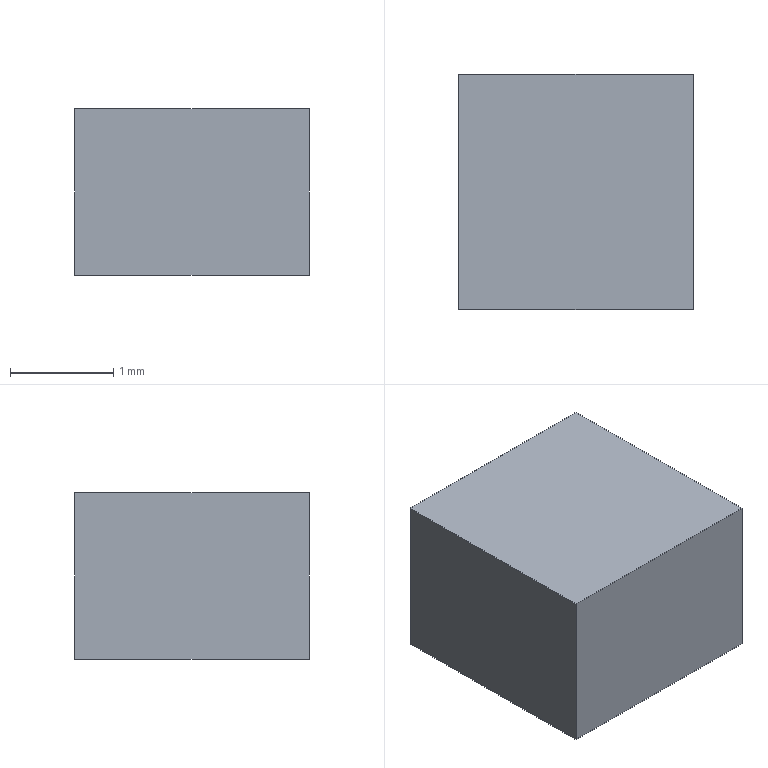Part | Creo | 1 solid | 6 faces | box 2.272 x 2.272 x 1.606 mm | volume 8.291 mm3 | plane 6
STEP:
#1=CARTESIAN_POINT('',(0.,0.,0.));
#2=DIRECTION('',(0.,0.,1.));
#3=DIRECTION('',(1.,0.,0.));
#4=AXIS2_PLACEMENT_3D('',#1,#2,#3);
#5=CARTESIAN_POINT('',(-1.136,-1.136,0.));
#6=VERTEX_POINT('',#5);
#7=CARTESIAN_POINT('',(1.136,-1.136,0.));
#8=VERTEX_POINT('',#7);
#9=CARTESIAN_POINT('',(-1.136,-1.136,0.));
#10=DIRECTION('',(1.,0.,0.));
#11=VECTOR('',#10,2.272);
#12=LINE('',#9,#11);
#13=EDGE_CURVE('',#6,#8,#12,.T.);
#14=ORIENTED_EDGE('',*,*,#13,.T.);
#15=CARTESIAN_POINT('',(1.136,1.136,0.));
#16=VERTEX_POINT('',#15);
#17=CARTESIAN_POINT('',(1.136,-1.136,0.));
#18=DIRECTION('',(0.,1.,0.));
#19=VECTOR('',#18,2.272);
#20=LINE('',#17,#19);
#21=EDGE_CURVE('',#8,#16,#20,.T.);
#22=ORIENTED_EDGE('',*,*,#21,.T.);
#23=CARTESIAN_POINT('',(-1.136,1.136,0.));
#24=VERTEX_POINT('',#23);
#25=CARTESIAN_POINT('',(1.136,1.136,0.));
#26=DIRECTION('',(-1.,0.,0.));
#27=VECTOR('',#26,2.272);
#28=LINE('',#25,#27);
#29=EDGE_CURVE('',#16,#24,#28,.T.);
#30=ORIENTED_EDGE('',*,*,#29,.T.);
#31=CARTESIAN_POINT('',(-1.136,1.136,0.));
#32=DIRECTION('',(0.,-1.,0.));
#33=VECTOR('',#32,2.272);
#34=LINE('',#31,#33);
#35=EDGE_CURVE('',#24,#6,#34,.T.);
#36=ORIENTED_EDGE('',*,*,#35,.T.);
#37=EDGE_LOOP('',(#14,#22,#30,#36));
#38=FACE_OUTER_BOUND('',#37,.F.);
#39=CARTESIAN_POINT('',(0.,0.,0.));
#40=DIRECTION('',(0.,0.,1.));
#41=DIRECTION('',(1.,0.,0.));
#42=AXIS2_PLACEMENT_3D('',#39,#40,#41);
#43=PLANE('',#42);
#44=ADVANCED_FACE('',(#38),#43,.F.);
#45=ORIENTED_EDGE('',*,*,#13,.F.);
#46=CARTESIAN_POINT('',(-1.136,-1.136,1.606));
#47=VERTEX_POINT('',#46);
#48=CARTESIAN_POINT('',(-1.136,-1.136,0.));
#49=DIRECTION('',(0.,0.,1.));
#50=VECTOR('',#49,1.606);
#51=LINE('',#48,#50);
#52=EDGE_CURVE('',#6,#47,#51,.T.);
#53=ORIENTED_EDGE('',*,*,#52,.T.);
#54=CARTESIAN_POINT('',(1.136,-1.136,1.606));
#55=VERTEX_POINT('',#54);
#56=CARTESIAN_POINT('',(-1.136,-1.136,1.606));
#57=DIRECTION('',(1.,0.,0.));
#58=VECTOR('',#57,2.272);
#59=LINE('',#56,#58);
#60=EDGE_CURVE('',#47,#55,#59,.T.);
#61=ORIENTED_EDGE('',*,*,#60,.T.);
#62=CARTESIAN_POINT('',(1.136,-1.136,0.));
#63=DIRECTION('',(0.,0.,1.));
#64=VECTOR('',#63,1.606);
#65=LINE('',#62,#64);
#66=EDGE_CURVE('',#8,#55,#65,.T.);
#67=ORIENTED_EDGE('',*,*,#66,.F.);
#68=EDGE_LOOP('',(#45,#53,#61,#67));
#69=FACE_OUTER_BOUND('',#68,.F.);
#70=CARTESIAN_POINT('',(-1.136,-1.136,0.));
#71=DIRECTION('',(0.,-1.,0.));
#72=DIRECTION('',(1.,0.,0.));
#73=AXIS2_PLACEMENT_3D('',#70,#71,#72);
#74=PLANE('',#73);
#75=ADVANCED_FACE('',(#69),#74,.T.);
#76=ORIENTED_EDGE('',*,*,#35,.F.);
#77=CARTESIAN_POINT('',(-1.136,1.136,1.606));
#78=VERTEX_POINT('',#77);
#79=CARTESIAN_POINT('',(-1.136,1.136,0.));
#80=DIRECTION('',(0.,0.,1.));
#81=VECTOR('',#80,1.606);
#82=LINE('',#79,#81);
#83=EDGE_CURVE('',#24,#78,#82,.T.);
#84=ORIENTED_EDGE('',*,*,#83,.T.);
#85=CARTESIAN_POINT('',(-1.136,1.136,1.606));
#86=DIRECTION('',(0.,-1.,0.));
#87=VECTOR('',#86,2.272);
#88=LINE('',#85,#87);
#89=EDGE_CURVE('',#78,#47,#88,.T.);
#90=ORIENTED_EDGE('',*,*,#89,.T.);
#91=ORIENTED_EDGE('',*,*,#52,.F.);
#92=EDGE_LOOP('',(#76,#84,#90,#91));
#93=FACE_OUTER_BOUND('',#92,.F.);
#94=CARTESIAN_POINT('',(-1.136,1.136,0.));
#95=DIRECTION('',(-1.,0.,0.));
#96=DIRECTION('',(0.,-1.,0.));
#97=AXIS2_PLACEMENT_3D('',#94,#95,#96);
#98=PLANE('',#97);
#99=ADVANCED_FACE('',(#93),#98,.T.);
#100=ORIENTED_EDGE('',*,*,#29,.F.);
#101=CARTESIAN_POINT('',(1.136,1.136,1.606));
#102=VERTEX_POINT('',#101);
#103=CARTESIAN_POINT('',(1.136,1.136,0.));
#104=DIRECTION('',(0.,0.,1.));
#105=VECTOR('',#104,1.606);
#106=LINE('',#103,#105);
#107=EDGE_CURVE('',#16,#102,#106,.T.);
#108=ORIENTED_EDGE('',*,*,#107,.T.);
#109=CARTESIAN_POINT('',(1.136,1.136,1.606));
#110=DIRECTION('',(-1.,0.,0.));
#111=VECTOR('',#110,2.272);
#112=LINE('',#109,#111);
#113=EDGE_CURVE('',#102,#78,#112,.T.);
#114=ORIENTED_EDGE('',*,*,#113,.T.);
#115=ORIENTED_EDGE('',*,*,#83,.F.);
#116=EDGE_LOOP('',(#100,#108,#114,#115));
#117=FACE_OUTER_BOUND('',#116,.F.);
#118=CARTESIAN_POINT('',(1.136,1.136,0.));
#119=DIRECTION('',(0.,1.,0.));
#120=DIRECTION('',(-1.,0.,0.));
#121=AXIS2_PLACEMENT_3D('',#118,#119,#120);
#122=PLANE('',#121);
#123=ADVANCED_FACE('',(#117),#122,.T.);
#124=ORIENTED_EDGE('',*,*,#21,.F.);
#125=ORIENTED_EDGE('',*,*,#66,.T.);
#126=CARTESIAN_POINT('',(1.136,-1.136,1.606));
#127=DIRECTION('',(0.,1.,0.));
#128=VECTOR('',#127,2.272);
#129=LINE('',#126,#128);
#130=EDGE_CURVE('',#55,#102,#129,.T.);
#131=ORIENTED_EDGE('',*,*,#130,.T.);
#132=ORIENTED_EDGE('',*,*,#107,.F.);
#133=EDGE_LOOP('',(#124,#125,#131,#132));
#134=FACE_OUTER_BOUND('',#133,.F.);
#135=CARTESIAN_POINT('',(1.136,-1.136,0.));
#136=DIRECTION('',(1.,0.,0.));
#137=DIRECTION('',(0.,1.,0.));
#138=AXIS2_PLACEMENT_3D('',#135,#136,#137);
#139=PLANE('',#138);
#140=ADVANCED_FACE('',(#134),#139,.T.);
#141=ORIENTED_EDGE('',*,*,#60,.F.);
#142=ORIENTED_EDGE('',*,*,#89,.F.);
#143=ORIENTED_EDGE('',*,*,#113,.F.);
#144=ORIENTED_EDGE('',*,*,#130,.F.);
#145=EDGE_LOOP('',(#141,#142,#143,#144));
#146=FACE_OUTER_BOUND('',#145,.F.);
#147=CARTESIAN_POINT('',(0.,0.,1.606));
#148=DIRECTION('',(0.,0.,1.));
#149=DIRECTION('',(1.,0.,0.));
#150=AXIS2_PLACEMENT_3D('',#147,#148,#149);
#151=PLANE('',#150);
#152=ADVANCED_FACE('',(#146),#151,.T.);
#153=CLOSED_SHELL('',(#44,#75,#99,#123,#140,#152));
#154=MANIFOLD_SOLID_BREP('',#153);
#155=(LENGTH_UNIT()NAMED_UNIT(*)SI_UNIT(.MILLI.,.METRE.));
#156=UNCERTAINTY_MEASURE_WITH_UNIT(LENGTH_MEASURE(0.0003592),#155,'','');
#157=(NAMED_UNIT(*)PLANE_ANGLE_UNIT()SI_UNIT($,.RADIAN.));
#158=PLANE_ANGLE_MEASURE_WITH_UNIT(PLANE_ANGLE_MEASURE(0.01745),#157);
#159=(CONVERSION_BASED_UNIT('DEGREE',#158)NAMED_UNIT(*)PLANE_ANGLE_UNIT());
#160=(NAMED_UNIT(*)SI_UNIT($,.STERADIAN.)SOLID_ANGLE_UNIT());
#161=(GEOMETRIC_REPRESENTATION_CONTEXT(3)GLOBAL_UNCERTAINTY_ASSIGNED_CONTEXT((#156))GLOBAL_UNIT_ASSIGNED_CONTEXT((#155,#159,#160))REPRESENTATION_CONTEXT('',''));
#162=ADVANCED_BREP_SHAPE_REPRESENTATION('',(#4,#154),#161);